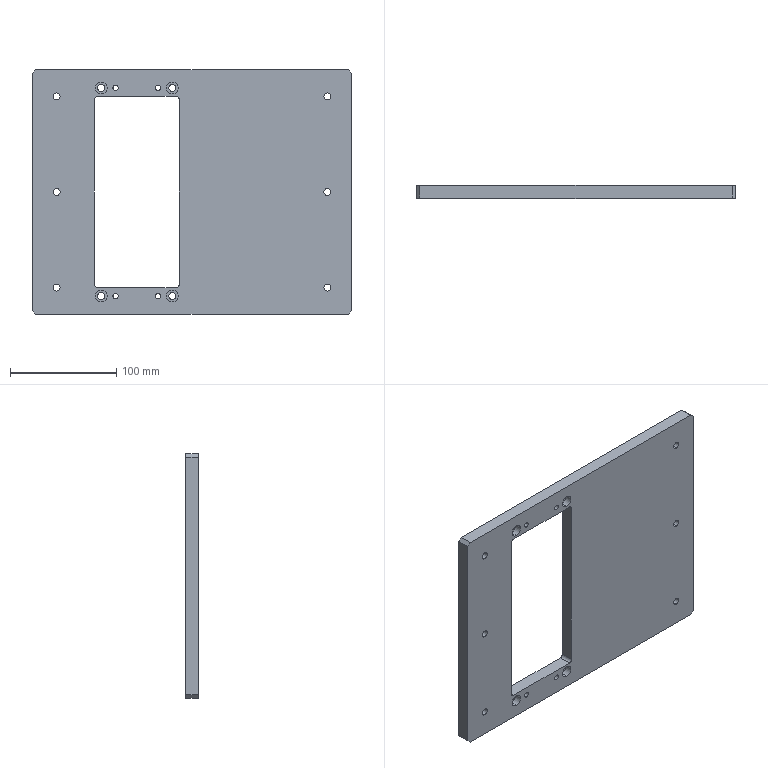Part | STEP file | PN_0021 | 1 solid | 76 faces | box 300 x 12 x 230 mm | volume 646136 mm3 | cylinder 52 | plane 24 | commonest cylinder face diameters 6.6 x20 11 x20 5 x8 6 x4